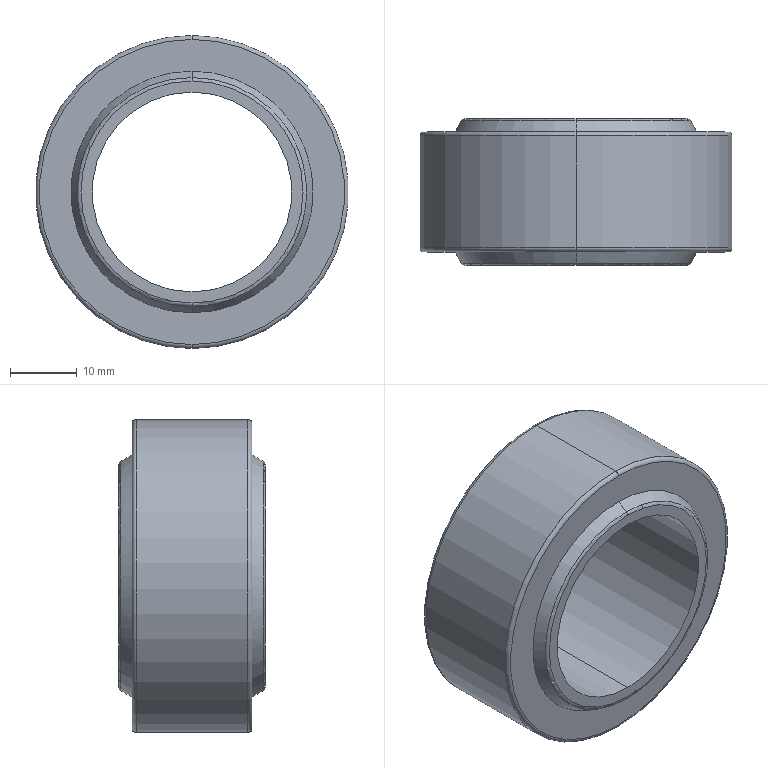Part | SolidWorks | features Revolution 2 | 1 solid | 20 faces | box 47 x 22 x 47 mm | volume 19543 mm3 | torus 8 | cylinder 4 | sphere 4 | plane 4 | commonest cylinder face diameters 30 x2 47 x2
STEP:
#1=CARTESIAN_POINT('',(0.,-11.,-15.));
#2=VERTEX_POINT('',#1);
#3=CARTESIAN_POINT('',(0.,-11.,15.));
#4=VERTEX_POINT('',#3);
#5=CARTESIAN_POINT('',(0.,-11.,0.));
#6=DIRECTION('',(0.,1.,0.));
#7=DIRECTION('',(0.,0.,1.));
#8=AXIS2_PLACEMENT_3D('',#5,#6,#7);
#9=CIRCLE('',#8,15.);
#10=EDGE_CURVE('',#2,#4,#9,.T.);
#11=ORIENTED_EDGE('',*,*,#10,.F.);
#12=CARTESIAN_POINT('',(0.,11.,-15.));
#13=VERTEX_POINT('',#12);
#14=CARTESIAN_POINT('',(0.,11.,-15.));
#15=DIRECTION('',(0.,1.,0.));
#16=VECTOR('',#15,1000.);
#17=LINE('',#14,#16);
#18=EDGE_CURVE('',#2,#13,#17,.T.);
#19=ORIENTED_EDGE('',*,*,#18,.T.);
#20=CARTESIAN_POINT('',(0.,11.,15.));
#21=VERTEX_POINT('',#20);
#22=CARTESIAN_POINT('',(0.,11.,0.));
#23=DIRECTION('',(0.,1.,0.));
#24=DIRECTION('',(0.,0.,1.));
#25=AXIS2_PLACEMENT_3D('',#22,#23,#24);
#26=CIRCLE('',#25,15.);
#27=EDGE_CURVE('',#13,#21,#26,.T.);
#28=ORIENTED_EDGE('',*,*,#27,.T.);
#29=CARTESIAN_POINT('',(0.,11.,15.));
#30=DIRECTION('',(0.,1.,0.));
#31=VECTOR('',#30,1000.);
#32=LINE('',#29,#31);
#33=EDGE_CURVE('',#4,#21,#32,.T.);
#34=ORIENTED_EDGE('',*,*,#33,.F.);
#35=EDGE_LOOP('',(#11,#19,#28,#34));
#36=FACE_OUTER_BOUND('',#35,.T.);
#37=CARTESIAN_POINT('',(0.,11.,0.));
#38=DIRECTION('',(0.,1.,0.));
#39=DIRECTION('',(0.,0.,1.));
#40=AXIS2_PLACEMENT_3D('',#37,#38,#39);
#41=CYLINDRICAL_SURFACE('',#40,15.);
#42=ADVANCED_FACE('',(#36),#41,.F.);
#43=CARTESIAN_POINT('',(0.,-11.,16.67));
#44=VERTEX_POINT('',#43);
#45=CARTESIAN_POINT('',(0.,-11.,-16.67));
#46=VERTEX_POINT('',#45);
#47=CARTESIAN_POINT('',(0.,-11.,0.));
#48=DIRECTION('',(0.,1.,0.));
#49=DIRECTION('',(0.,0.,1.));
#50=AXIS2_PLACEMENT_3D('',#47,#48,#49);
#51=CIRCLE('',#50,16.67);
#52=EDGE_CURVE('',#44,#46,#51,.T.);
#53=ORIENTED_EDGE('',*,*,#52,.T.);
#54=CARTESIAN_POINT('',(0.,-10.718,-17.179));
#55=VERTEX_POINT('',#54);
#56=CARTESIAN_POINT('',(0.,-10.4,-16.67));
#57=DIRECTION('',(1.,0.,0.));
#58=DIRECTION('',(0.,0.,-1.));
#59=AXIS2_PLACEMENT_3D('',#56,#57,#58);
#60=CIRCLE('',#59,0.6);
#61=EDGE_CURVE('',#46,#55,#60,.T.);
#62=ORIENTED_EDGE('',*,*,#61,.T.);
#63=CARTESIAN_POINT('',(0.,-10.718,17.179));
#64=VERTEX_POINT('',#63);
#65=CARTESIAN_POINT('',(0.,-10.718,0.));
#66=DIRECTION('',(0.,1.,0.));
#67=DIRECTION('',(0.,0.,1.));
#68=AXIS2_PLACEMENT_3D('',#65,#66,#67);
#69=CIRCLE('',#68,17.179);
#70=EDGE_CURVE('',#64,#55,#69,.T.);
#71=ORIENTED_EDGE('',*,*,#70,.F.);
#72=CARTESIAN_POINT('',(0.,-10.4,16.67));
#73=DIRECTION('',(-1.,0.,0.));
#74=DIRECTION('',(0.,0.,1.));
#75=AXIS2_PLACEMENT_3D('',#72,#73,#74);
#76=CIRCLE('',#75,0.6);
#77=EDGE_CURVE('',#44,#64,#76,.T.);
#78=ORIENTED_EDGE('',*,*,#77,.F.);
#79=EDGE_LOOP('',(#53,#62,#71,#78));
#80=FACE_OUTER_BOUND('',#79,.T.);
#81=CARTESIAN_POINT('',(0.,-10.4,0.));
#82=DIRECTION('',(0.,1.,0.));
#83=DIRECTION('',(0.,0.,1.));
#84=AXIS2_PLACEMENT_3D('',#81,#82,#83);
#85=TOROIDAL_SURFACE('',#84,16.67,0.6);
#86=ADVANCED_FACE('',(#80),#85,.T.);
#87=CARTESIAN_POINT('',(0.,9.,18.138));
#88=VERTEX_POINT('',#87);
#89=CARTESIAN_POINT('',(0.,9.,-18.138));
#90=VERTEX_POINT('',#89);
#91=CARTESIAN_POINT('',(0.,9.,0.));
#92=DIRECTION('',(0.,1.,0.));
#93=DIRECTION('',(0.,0.,1.));
#94=AXIS2_PLACEMENT_3D('',#91,#92,#93);
#95=CIRCLE('',#94,18.138);
#96=EDGE_CURVE('',#88,#90,#95,.T.);
#97=ORIENTED_EDGE('',*,*,#96,.T.);
#98=CARTESIAN_POINT('',(0.,10.718,-17.179));
#99=VERTEX_POINT('',#98);
#100=CARTESIAN_POINT('',(0.,0.,0.));
#101=DIRECTION('',(1.,0.,0.));
#102=DIRECTION('',(0.,0.,-1.));
#103=AXIS2_PLACEMENT_3D('',#100,#101,#102);
#104=CIRCLE('',#103,20.248);
#105=EDGE_CURVE('',#90,#99,#104,.T.);
#106=ORIENTED_EDGE('',*,*,#105,.T.);
#107=CARTESIAN_POINT('',(0.,10.718,17.179));
#108=VERTEX_POINT('',#107);
#109=CARTESIAN_POINT('',(0.,10.718,0.));
#110=DIRECTION('',(0.,1.,0.));
#111=DIRECTION('',(0.,0.,1.));
#112=AXIS2_PLACEMENT_3D('',#109,#110,#111);
#113=CIRCLE('',#112,17.179);
#114=EDGE_CURVE('',#108,#99,#113,.T.);
#115=ORIENTED_EDGE('',*,*,#114,.F.);
#116=CARTESIAN_POINT('',(0.,0.,0.));
#117=DIRECTION('',(-1.,0.,0.));
#118=DIRECTION('',(0.,0.,1.));
#119=AXIS2_PLACEMENT_3D('',#116,#117,#118);
#120=CIRCLE('',#119,20.248);
#121=EDGE_CURVE('',#88,#108,#120,.T.);
#122=ORIENTED_EDGE('',*,*,#121,.F.);
#123=EDGE_LOOP('',(#97,#106,#115,#122));
#124=FACE_OUTER_BOUND('',#123,.T.);
#125=CARTESIAN_POINT('',(0.,0.,0.));
#126=DIRECTION('',(1.,0.,0.));
#127=DIRECTION('',(0.,0.,1.));
#128=AXIS2_PLACEMENT_3D('',#125,#126,#127);
#129=SPHERICAL_SURFACE('',#128,20.248);
#130=ADVANCED_FACE('',(#124),#129,.T.);
#131=ORIENTED_EDGE('',*,*,#114,.T.);
#132=CARTESIAN_POINT('',(0.,11.,-16.67));
#133=VERTEX_POINT('',#132);
#134=CARTESIAN_POINT('',(0.,10.4,-16.67));
#135=DIRECTION('',(1.,0.,0.));
#136=DIRECTION('',(0.,0.,-1.));
#137=AXIS2_PLACEMENT_3D('',#134,#135,#136);
#138=CIRCLE('',#137,0.6);
#139=EDGE_CURVE('',#99,#133,#138,.T.);
#140=ORIENTED_EDGE('',*,*,#139,.T.);
#141=CARTESIAN_POINT('',(0.,11.,16.67));
#142=VERTEX_POINT('',#141);
#143=CARTESIAN_POINT('',(0.,11.,0.));
#144=DIRECTION('',(0.,1.,0.));
#145=DIRECTION('',(0.,0.,1.));
#146=AXIS2_PLACEMENT_3D('',#143,#144,#145);
#147=CIRCLE('',#146,16.67);
#148=EDGE_CURVE('',#142,#133,#147,.T.);
#149=ORIENTED_EDGE('',*,*,#148,.F.);
#150=CARTESIAN_POINT('',(0.,10.4,16.67));
#151=DIRECTION('',(-1.,0.,0.));
#152=DIRECTION('',(0.,0.,1.));
#153=AXIS2_PLACEMENT_3D('',#150,#151,#152);
#154=CIRCLE('',#153,0.6);
#155=EDGE_CURVE('',#108,#142,#154,.T.);
#156=ORIENTED_EDGE('',*,*,#155,.F.);
#157=EDGE_LOOP('',(#131,#140,#149,#156));
#158=FACE_OUTER_BOUND('',#157,.T.);
#159=CARTESIAN_POINT('',(0.,10.4,0.));
#160=DIRECTION('',(0.,1.,0.));
#161=DIRECTION('',(0.,0.,1.));
#162=AXIS2_PLACEMENT_3D('',#159,#160,#161);
#163=TOROIDAL_SURFACE('',#162,16.67,0.6);
#164=ADVANCED_FACE('',(#158),#163,.T.);
#165=ORIENTED_EDGE('',*,*,#70,.T.);
#166=CARTESIAN_POINT('',(0.,-9.,-18.138));
#167=VERTEX_POINT('',#166);
#168=CARTESIAN_POINT('',(0.,0.,0.));
#169=DIRECTION('',(1.,0.,0.));
#170=DIRECTION('',(0.,0.,-1.));
#171=AXIS2_PLACEMENT_3D('',#168,#169,#170);
#172=CIRCLE('',#171,20.248);
#173=EDGE_CURVE('',#55,#167,#172,.T.);
#174=ORIENTED_EDGE('',*,*,#173,.T.);
#175=CARTESIAN_POINT('',(0.,-9.,18.138));
#176=VERTEX_POINT('',#175);
#177=CARTESIAN_POINT('',(0.,-9.,0.));
#178=DIRECTION('',(0.,-1.,0.));
#179=DIRECTION('',(0.,0.,-1.));
#180=AXIS2_PLACEMENT_3D('',#177,#178,#179);
#181=CIRCLE('',#180,18.138);
#182=EDGE_CURVE('',#167,#176,#181,.T.);
#183=ORIENTED_EDGE('',*,*,#182,.T.);
#184=CARTESIAN_POINT('',(0.,0.,0.));
#185=DIRECTION('',(-1.,0.,0.));
#186=DIRECTION('',(0.,0.,1.));
#187=AXIS2_PLACEMENT_3D('',#184,#185,#186);
#188=CIRCLE('',#187,20.248);
#189=EDGE_CURVE('',#64,#176,#188,.T.);
#190=ORIENTED_EDGE('',*,*,#189,.F.);
#191=EDGE_LOOP('',(#165,#174,#183,#190));
#192=FACE_OUTER_BOUND('',#191,.T.);
#193=CARTESIAN_POINT('',(0.,0.,0.));
#194=DIRECTION('',(1.,0.,0.));
#195=DIRECTION('',(0.,0.,1.));
#196=AXIS2_PLACEMENT_3D('',#193,#194,#195);
#197=SPHERICAL_SURFACE('',#196,20.248);
#198=ADVANCED_FACE('',(#192),#197,.T.);
#199=CARTESIAN_POINT('',(0.,-9.,22.9));
#200=VERTEX_POINT('',#199);
#201=CARTESIAN_POINT('',(0.,-9.,-22.9));
#202=VERTEX_POINT('',#201);
#203=CARTESIAN_POINT('',(0.,-9.,0.));
#204=DIRECTION('',(0.,1.,0.));
#205=DIRECTION('',(0.,0.,1.));
#206=AXIS2_PLACEMENT_3D('',#203,#204,#205);
#207=CIRCLE('',#206,22.9);
#208=EDGE_CURVE('',#200,#202,#207,.T.);
#209=ORIENTED_EDGE('',*,*,#208,.T.);
#210=CARTESIAN_POINT('',(0.,-8.4,-23.5));
#211=VERTEX_POINT('',#210);
#212=CARTESIAN_POINT('',(0.,-8.4,-22.9));
#213=DIRECTION('',(1.,0.,0.));
#214=DIRECTION('',(0.,0.,-1.));
#215=AXIS2_PLACEMENT_3D('',#212,#213,#214);
#216=CIRCLE('',#215,0.6);
#217=EDGE_CURVE('',#202,#211,#216,.T.);
#218=ORIENTED_EDGE('',*,*,#217,.T.);
#219=CARTESIAN_POINT('',(0.,-8.4,23.5));
#220=VERTEX_POINT('',#219);
#221=CARTESIAN_POINT('',(0.,-8.4,0.));
#222=DIRECTION('',(0.,1.,0.));
#223=DIRECTION('',(0.,0.,1.));
#224=AXIS2_PLACEMENT_3D('',#221,#222,#223);
#225=CIRCLE('',#224,23.5);
#226=EDGE_CURVE('',#220,#211,#225,.T.);
#227=ORIENTED_EDGE('',*,*,#226,.F.);
#228=CARTESIAN_POINT('',(0.,-8.4,22.9));
#229=DIRECTION('',(-1.,0.,0.));
#230=DIRECTION('',(0.,0.,1.));
#231=AXIS2_PLACEMENT_3D('',#228,#229,#230);
#232=CIRCLE('',#231,0.6);
#233=EDGE_CURVE('',#200,#220,#232,.T.);
#234=ORIENTED_EDGE('',*,*,#233,.F.);
#235=EDGE_LOOP('',(#209,#218,#227,#234));
#236=FACE_OUTER_BOUND('',#235,.T.);
#237=CARTESIAN_POINT('',(0.,-8.4,0.));
#238=DIRECTION('',(0.,1.,0.));
#239=DIRECTION('',(0.,0.,1.));
#240=AXIS2_PLACEMENT_3D('',#237,#238,#239);
#241=TOROIDAL_SURFACE('',#240,22.9,0.6);
#242=ADVANCED_FACE('',(#236),#241,.T.);
#243=ORIENTED_EDGE('',*,*,#226,.T.);
#244=CARTESIAN_POINT('',(0.,8.4,-23.5));
#245=VERTEX_POINT('',#244);
#246=CARTESIAN_POINT('',(0.,11.,-23.5));
#247=DIRECTION('',(0.,1.,0.));
#248=VECTOR('',#247,1000.);
#249=LINE('',#246,#248);
#250=EDGE_CURVE('',#211,#245,#249,.T.);
#251=ORIENTED_EDGE('',*,*,#250,.T.);
#252=CARTESIAN_POINT('',(0.,8.4,23.5));
#253=VERTEX_POINT('',#252);
#254=CARTESIAN_POINT('',(0.,8.4,0.));
#255=DIRECTION('',(0.,1.,0.));
#256=DIRECTION('',(0.,0.,1.));
#257=AXIS2_PLACEMENT_3D('',#254,#255,#256);
#258=CIRCLE('',#257,23.5);
#259=EDGE_CURVE('',#253,#245,#258,.T.);
#260=ORIENTED_EDGE('',*,*,#259,.F.);
#261=CARTESIAN_POINT('',(0.,11.,23.5));
#262=DIRECTION('',(0.,1.,0.));
#263=VECTOR('',#262,1000.);
#264=LINE('',#261,#263);
#265=EDGE_CURVE('',#220,#253,#264,.T.);
#266=ORIENTED_EDGE('',*,*,#265,.F.);
#267=EDGE_LOOP('',(#243,#251,#260,#266));
#268=FACE_OUTER_BOUND('',#267,.T.);
#269=CARTESIAN_POINT('',(0.,11.,0.));
#270=DIRECTION('',(0.,1.,0.));
#271=DIRECTION('',(0.,0.,1.));
#272=AXIS2_PLACEMENT_3D('',#269,#270,#271);
#273=CYLINDRICAL_SURFACE('',#272,23.5);
#274=ADVANCED_FACE('',(#268),#273,.T.);
#275=ORIENTED_EDGE('',*,*,#259,.T.);
#276=CARTESIAN_POINT('',(0.,9.,-22.9));
#277=VERTEX_POINT('',#276);
#278=CARTESIAN_POINT('',(0.,8.4,-22.9));
#279=DIRECTION('',(1.,0.,0.));
#280=DIRECTION('',(0.,0.,-1.));
#281=AXIS2_PLACEMENT_3D('',#278,#279,#280);
#282=CIRCLE('',#281,0.6);
#283=EDGE_CURVE('',#245,#277,#282,.T.);
#284=ORIENTED_EDGE('',*,*,#283,.T.);
#285=CARTESIAN_POINT('',(0.,9.,22.9));
#286=VERTEX_POINT('',#285);
#287=CARTESIAN_POINT('',(0.,9.,0.));
#288=DIRECTION('',(0.,1.,0.));
#289=DIRECTION('',(0.,0.,1.));
#290=AXIS2_PLACEMENT_3D('',#287,#288,#289);
#291=CIRCLE('',#290,22.9);
#292=EDGE_CURVE('',#286,#277,#291,.T.);
#293=ORIENTED_EDGE('',*,*,#292,.F.);
#294=CARTESIAN_POINT('',(0.,8.4,22.9));
#295=DIRECTION('',(-1.,0.,0.));
#296=DIRECTION('',(0.,0.,1.));
#297=AXIS2_PLACEMENT_3D('',#294,#295,#296);
#298=CIRCLE('',#297,0.6);
#299=EDGE_CURVE('',#253,#286,#298,.T.);
#300=ORIENTED_EDGE('',*,*,#299,.F.);
#301=EDGE_LOOP('',(#275,#284,#293,#300));
#302=FACE_OUTER_BOUND('',#301,.T.);
#303=CARTESIAN_POINT('',(0.,8.4,0.));
#304=DIRECTION('',(0.,1.,0.));
#305=DIRECTION('',(0.,0.,1.));
#306=AXIS2_PLACEMENT_3D('',#303,#304,#305);
#307=TOROIDAL_SURFACE('',#306,22.9,0.6);
#308=ADVANCED_FACE('',(#302),#307,.T.);
#309=ORIENTED_EDGE('',*,*,#283,.F.);
#310=CARTESIAN_POINT('',(0.,8.4,0.));
#311=DIRECTION('',(0.,1.,0.));
#312=DIRECTION('',(0.,0.,1.));
#313=AXIS2_PLACEMENT_3D('',#310,#311,#312);
#314=CIRCLE('',#313,23.5);
#315=EDGE_CURVE('',#245,#253,#314,.T.);
#316=ORIENTED_EDGE('',*,*,#315,.T.);
#317=ORIENTED_EDGE('',*,*,#299,.T.);
#318=CARTESIAN_POINT('',(0.,9.,0.));
#319=DIRECTION('',(0.,1.,0.));
#320=DIRECTION('',(0.,0.,1.));
#321=AXIS2_PLACEMENT_3D('',#318,#319,#320);
#322=CIRCLE('',#321,22.9);
#323=EDGE_CURVE('',#277,#286,#322,.T.);
#324=ORIENTED_EDGE('',*,*,#323,.F.);
#325=EDGE_LOOP('',(#309,#316,#317,#324));
#326=FACE_OUTER_BOUND('',#325,.T.);
#327=CARTESIAN_POINT('',(0.,8.4,0.));
#328=DIRECTION('',(0.,1.,0.));
#329=DIRECTION('',(0.,0.,1.));
#330=AXIS2_PLACEMENT_3D('',#327,#328,#329);
#331=TOROIDAL_SURFACE('',#330,22.9,0.6);
#332=ADVANCED_FACE('',(#326),#331,.T.);
#333=ORIENTED_EDGE('',*,*,#250,.F.);
#334=CARTESIAN_POINT('',(0.,-8.4,0.));
#335=DIRECTION('',(0.,1.,0.));
#336=DIRECTION('',(0.,0.,1.));
#337=AXIS2_PLACEMENT_3D('',#334,#335,#336);
#338=CIRCLE('',#337,23.5);
#339=EDGE_CURVE('',#211,#220,#338,.T.);
#340=ORIENTED_EDGE('',*,*,#339,.T.);
#341=ORIENTED_EDGE('',*,*,#265,.T.);
#342=ORIENTED_EDGE('',*,*,#315,.F.);
#343=EDGE_LOOP('',(#333,#340,#341,#342));
#344=FACE_OUTER_BOUND('',#343,.T.);
#345=CARTESIAN_POINT('',(0.,11.,0.));
#346=DIRECTION('',(0.,1.,0.));
#347=DIRECTION('',(0.,0.,1.));
#348=AXIS2_PLACEMENT_3D('',#345,#346,#347);
#349=CYLINDRICAL_SURFACE('',#348,23.5);
#350=ADVANCED_FACE('',(#344),#349,.T.);
#351=ORIENTED_EDGE('',*,*,#217,.F.);
#352=CARTESIAN_POINT('',(0.,-9.,0.));
#353=DIRECTION('',(0.,1.,0.));
#354=DIRECTION('',(0.,0.,1.));
#355=AXIS2_PLACEMENT_3D('',#352,#353,#354);
#356=CIRCLE('',#355,22.9);
#357=EDGE_CURVE('',#202,#200,#356,.T.);
#358=ORIENTED_EDGE('',*,*,#357,.T.);
#359=ORIENTED_EDGE('',*,*,#233,.T.);
#360=ORIENTED_EDGE('',*,*,#339,.F.);
#361=EDGE_LOOP('',(#351,#358,#359,#360));
#362=FACE_OUTER_BOUND('',#361,.T.);
#363=CARTESIAN_POINT('',(0.,-8.4,0.));
#364=DIRECTION('',(0.,1.,0.));
#365=DIRECTION('',(0.,0.,1.));
#366=AXIS2_PLACEMENT_3D('',#363,#364,#365);
#367=TOROIDAL_SURFACE('',#366,22.9,0.6);
#368=ADVANCED_FACE('',(#362),#367,.T.);
#369=CARTESIAN_POINT('',(0.,-9.,0.));
#370=DIRECTION('',(0.,-1.,0.));
#371=DIRECTION('',(0.,0.,-1.));
#372=AXIS2_PLACEMENT_3D('',#369,#370,#371);
#373=CIRCLE('',#372,18.138);
#374=EDGE_CURVE('',#176,#167,#373,.T.);
#375=ORIENTED_EDGE('',*,*,#374,.F.);
#376=ORIENTED_EDGE('',*,*,#182,.F.);
#377=EDGE_LOOP('',(#375,#376));
#378=FACE_BOUND('',#377,.T.);
#379=ORIENTED_EDGE('',*,*,#208,.F.);
#380=ORIENTED_EDGE('',*,*,#357,.F.);
#381=EDGE_LOOP('',(#379,#380));
#382=FACE_OUTER_BOUND('',#381,.T.);
#383=CARTESIAN_POINT('',(0.,-9.,22.9));
#384=DIRECTION('',(0.,-1.,0.));
#385=DIRECTION('',(0.,0.,-1.));
#386=AXIS2_PLACEMENT_3D('',#383,#384,#385);
#387=PLANE('',#386);
#388=ADVANCED_FACE('',(#378,#382),#387,.T.);
#389=ORIENTED_EDGE('',*,*,#292,.T.);
#390=ORIENTED_EDGE('',*,*,#323,.T.);
#391=EDGE_LOOP('',(#389,#390));
#392=FACE_OUTER_BOUND('',#391,.T.);
#393=ORIENTED_EDGE('',*,*,#96,.F.);
#394=CARTESIAN_POINT('',(0.,9.,0.));
#395=DIRECTION('',(0.,1.,0.));
#396=DIRECTION('',(0.,0.,1.));
#397=AXIS2_PLACEMENT_3D('',#394,#395,#396);
#398=CIRCLE('',#397,18.138);
#399=EDGE_CURVE('',#90,#88,#398,.T.);
#400=ORIENTED_EDGE('',*,*,#399,.F.);
#401=EDGE_LOOP('',(#393,#400));
#402=FACE_BOUND('',#401,.T.);
#403=CARTESIAN_POINT('',(0.,9.,22.9));
#404=DIRECTION('',(0.,1.,0.));
#405=DIRECTION('',(0.,0.,1.));
#406=AXIS2_PLACEMENT_3D('',#403,#404,#405);
#407=PLANE('',#406);
#408=ADVANCED_FACE('',(#392,#402),#407,.T.);
#409=ORIENTED_EDGE('',*,*,#173,.F.);
#410=CARTESIAN_POINT('',(0.,-10.718,0.));
#411=DIRECTION('',(0.,1.,0.));
#412=DIRECTION('',(0.,0.,1.));
#413=AXIS2_PLACEMENT_3D('',#410,#411,#412);
#414=CIRCLE('',#413,17.179);
#415=EDGE_CURVE('',#55,#64,#414,.T.);
#416=ORIENTED_EDGE('',*,*,#415,.T.);
#417=ORIENTED_EDGE('',*,*,#189,.T.);
#418=ORIENTED_EDGE('',*,*,#374,.T.);
#419=EDGE_LOOP('',(#409,#416,#417,#418));
#420=FACE_OUTER_BOUND('',#419,.T.);
#421=CARTESIAN_POINT('',(0.,0.,0.));
#422=DIRECTION('',(1.,0.,0.));
#423=DIRECTION('',(0.,0.,1.));
#424=AXIS2_PLACEMENT_3D('',#421,#422,#423);
#425=SPHERICAL_SURFACE('',#424,20.248);
#426=ADVANCED_FACE('',(#420),#425,.T.);
#427=ORIENTED_EDGE('',*,*,#139,.F.);
#428=CARTESIAN_POINT('',(0.,10.718,0.));
#429=DIRECTION('',(0.,1.,0.));
#430=DIRECTION('',(0.,0.,1.));
#431=AXIS2_PLACEMENT_3D('',#428,#429,#430);
#432=CIRCLE('',#431,17.179);
#433=EDGE_CURVE('',#99,#108,#432,.T.);
#434=ORIENTED_EDGE('',*,*,#433,.T.);
#435=ORIENTED_EDGE('',*,*,#155,.T.);
#436=CARTESIAN_POINT('',(0.,11.,0.));
#437=DIRECTION('',(0.,1.,0.));
#438=DIRECTION('',(0.,0.,1.));
#439=AXIS2_PLACEMENT_3D('',#436,#437,#438);
#440=CIRCLE('',#439,16.67);
#441=EDGE_CURVE('',#133,#142,#440,.T.);
#442=ORIENTED_EDGE('',*,*,#441,.F.);
#443=EDGE_LOOP('',(#427,#434,#435,#442));
#444=FACE_OUTER_BOUND('',#443,.T.);
#445=CARTESIAN_POINT('',(0.,10.4,0.));
#446=DIRECTION('',(0.,1.,0.));
#447=DIRECTION('',(0.,0.,1.));
#448=AXIS2_PLACEMENT_3D('',#445,#446,#447);
#449=TOROIDAL_SURFACE('',#448,16.67,0.6);
#450=ADVANCED_FACE('',(#444),#449,.T.);
#451=ORIENTED_EDGE('',*,*,#105,.F.);
#452=ORIENTED_EDGE('',*,*,#399,.T.);
#453=ORIENTED_EDGE('',*,*,#121,.T.);
#454=ORIENTED_EDGE('',*,*,#433,.F.);
#455=EDGE_LOOP('',(#451,#452,#453,#454));
#456=FACE_OUTER_BOUND('',#455,.T.);
#457=CARTESIAN_POINT('',(0.,0.,0.));
#458=DIRECTION('',(1.,0.,0.));
#459=DIRECTION('',(0.,0.,1.));
#460=AXIS2_PLACEMENT_3D('',#457,#458,#459);
#461=SPHERICAL_SURFACE('',#460,20.248);
#462=ADVANCED_FACE('',(#456),#461,.T.);
#463=ORIENTED_EDGE('',*,*,#61,.F.);
#464=CARTESIAN_POINT('',(0.,-11.,0.));
#465=DIRECTION('',(0.,1.,0.));
#466=DIRECTION('',(0.,0.,1.));
#467=AXIS2_PLACEMENT_3D('',#464,#465,#466);
#468=CIRCLE('',#467,16.67);
#469=EDGE_CURVE('',#46,#44,#468,.T.);
#470=ORIENTED_EDGE('',*,*,#469,.T.);
#471=ORIENTED_EDGE('',*,*,#77,.T.);
#472=ORIENTED_EDGE('',*,*,#415,.F.);
#473=EDGE_LOOP('',(#463,#470,#471,#472));
#474=FACE_OUTER_BOUND('',#473,.T.);
#475=CARTESIAN_POINT('',(0.,-10.4,0.));
#476=DIRECTION('',(0.,1.,0.));
#477=DIRECTION('',(0.,0.,1.));
#478=AXIS2_PLACEMENT_3D('',#475,#476,#477);
#479=TOROIDAL_SURFACE('',#478,16.67,0.6);
#480=ADVANCED_FACE('',(#474),#479,.T.);
#481=CARTESIAN_POINT('',(0.,-11.,0.));
#482=DIRECTION('',(0.,1.,0.));
#483=DIRECTION('',(0.,0.,1.));
#484=AXIS2_PLACEMENT_3D('',#481,#482,#483);
#485=CIRCLE('',#484,15.);
#486=EDGE_CURVE('',#4,#2,#485,.T.);
#487=ORIENTED_EDGE('',*,*,#486,.T.);
#488=ORIENTED_EDGE('',*,*,#10,.T.);
#489=EDGE_LOOP('',(#487,#488));
#490=FACE_BOUND('',#489,.T.);
#491=ORIENTED_EDGE('',*,*,#52,.F.);
#492=ORIENTED_EDGE('',*,*,#469,.F.);
#493=EDGE_LOOP('',(#491,#492));
#494=FACE_OUTER_BOUND('',#493,.T.);
#495=CARTESIAN_POINT('',(0.,-11.,16.67));
#496=DIRECTION('',(0.,-1.,0.));
#497=DIRECTION('',(0.,0.,-1.));
#498=AXIS2_PLACEMENT_3D('',#495,#496,#497);
#499=PLANE('',#498);
#500=ADVANCED_FACE('',(#490,#494),#499,.T.);
#501=ORIENTED_EDGE('',*,*,#18,.F.);
#502=ORIENTED_EDGE('',*,*,#486,.F.);
#503=ORIENTED_EDGE('',*,*,#33,.T.);
#504=CARTESIAN_POINT('',(0.,11.,0.));
#505=DIRECTION('',(0.,1.,0.));
#506=DIRECTION('',(0.,0.,1.));
#507=AXIS2_PLACEMENT_3D('',#504,#505,#506);
#508=CIRCLE('',#507,15.);
#509=EDGE_CURVE('',#21,#13,#508,.T.);
#510=ORIENTED_EDGE('',*,*,#509,.T.);
#511=EDGE_LOOP('',(#501,#502,#503,#510));
#512=FACE_OUTER_BOUND('',#511,.T.);
#513=CARTESIAN_POINT('',(0.,11.,0.));
#514=DIRECTION('',(0.,1.,0.));
#515=DIRECTION('',(0.,0.,1.));
#516=AXIS2_PLACEMENT_3D('',#513,#514,#515);
#517=CYLINDRICAL_SURFACE('',#516,15.);
#518=ADVANCED_FACE('',(#512),#517,.F.);
#519=ORIENTED_EDGE('',*,*,#148,.T.);
#520=ORIENTED_EDGE('',*,*,#441,.T.);
#521=EDGE_LOOP('',(#519,#520));
#522=FACE_OUTER_BOUND('',#521,.T.);
#523=ORIENTED_EDGE('',*,*,#509,.F.);
#524=ORIENTED_EDGE('',*,*,#27,.F.);
#525=EDGE_LOOP('',(#523,#524));
#526=FACE_BOUND('',#525,.T.);
#527=CARTESIAN_POINT('',(0.,11.,16.67));
#528=DIRECTION('',(0.,1.,0.));
#529=DIRECTION('',(0.,0.,1.));
#530=AXIS2_PLACEMENT_3D('',#527,#528,#529);
#531=PLANE('',#530);
#532=ADVANCED_FACE('',(#522,#526),#531,.T.);
#533=CLOSED_SHELL('',(#42,#86,#130,#164,#198,#242,#274,#308,#332,#350,#368,#388,#408,#426,#450,#462,#480,#500,#518,#532));
#534=MANIFOLD_SOLID_BREP('',#533);
#535=CARTESIAN_POINT('',(0.,0.,0.));
#536=DIRECTION('',(0.,0.,1.));
#537=DIRECTION('',(1.,0.,0.));
#538=AXIS2_PLACEMENT_3D('',#535,#536,#537);
#539=(LENGTH_UNIT()NAMED_UNIT(*)SI_UNIT(.MILLI.,.METRE.));
#540=UNCERTAINTY_MEASURE_WITH_UNIT(LENGTH_MEASURE(0.00001),#539,'','');
#541=(NAMED_UNIT(*)PLANE_ANGLE_UNIT()SI_UNIT($,.RADIAN.));
#542=(NAMED_UNIT(*)SI_UNIT($,.STERADIAN.)SOLID_ANGLE_UNIT());
#543=(GEOMETRIC_REPRESENTATION_CONTEXT(3)GLOBAL_UNCERTAINTY_ASSIGNED_CONTEXT((#540))GLOBAL_UNIT_ASSIGNED_CONTEXT((#539,#541,#542))REPRESENTATION_CONTEXT('',''));
#544=ADVANCED_BREP_SHAPE_REPRESENTATION('',(#534,#538),#543);